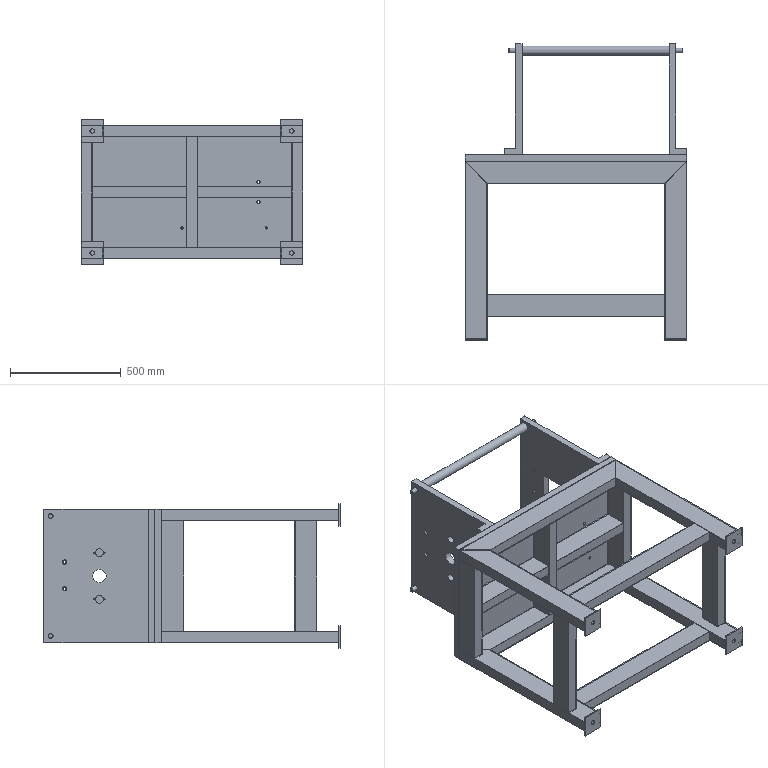Part | NX | features main frame_Default_As Machined_ 25 | 24 solids | 281 faces | box 1000 x 1335 x 650 mm | volume 44393432 mm3 | plane 212 | cylinder 51 | cone 18 | commonest cylinder face diameters 20 x16 22 x10 10.2 x6 14.5 x6 5 x4 13.5 x4